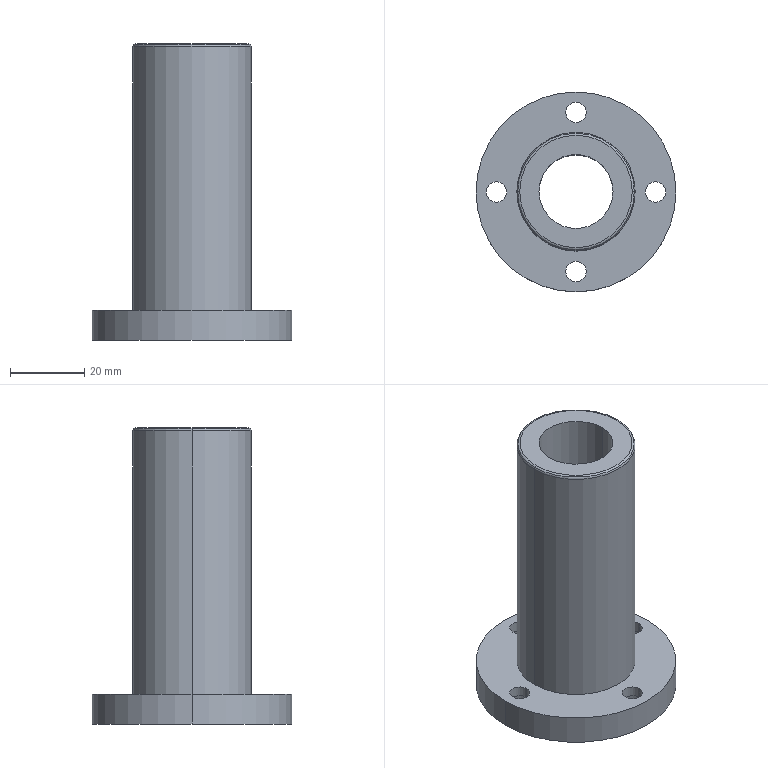Part | NX | features BREP 1 | 1 solid | 33 faces | box 54 x 54 x 80 mm | volume 49508 mm3 | cylinder 22 | plane 7 | torus 4 | commonest cylinder face diameters 5.5 x8 9 x8 20 x2 32 x2 54 x2
STEP:
#1=CARTESIAN_POINT('',(15.2,0.,80.));
#2=VERTEX_POINT('',#1);
#3=CARTESIAN_POINT('',(-15.2,0.,80.));
#4=VERTEX_POINT('',#3);
#5=CARTESIAN_POINT('',(0.,0.,80.));
#6=DIRECTION('',(0.,0.,1.));
#7=DIRECTION('',(1.,0.,0.));
#8=AXIS2_PLACEMENT_3D('',#5,#6,#7);
#9=CIRCLE('',#8,15.2);
#10=EDGE_CURVE('',#2,#4,#9,.T.);
#11=ORIENTED_EDGE('',*,*,#10,.T.);
#12=CARTESIAN_POINT('',(0.,0.,80.));
#13=DIRECTION('',(0.,0.,1.));
#14=DIRECTION('',(-1.,0.,0.));
#15=AXIS2_PLACEMENT_3D('',#12,#13,#14);
#16=CIRCLE('',#15,15.2);
#17=EDGE_CURVE('',#4,#2,#16,.T.);
#18=ORIENTED_EDGE('',*,*,#17,.T.);
#19=EDGE_LOOP('',(#11,#18));
#20=FACE_BOUND('',#19,.T.);
#21=CARTESIAN_POINT('',(10.,0.,80.));
#22=VERTEX_POINT('',#21);
#23=CARTESIAN_POINT('',(-10.,0.,80.));
#24=VERTEX_POINT('',#23);
#25=CARTESIAN_POINT('',(0.,0.,80.));
#26=DIRECTION('',(0.,0.,-1.));
#27=DIRECTION('',(1.,0.,0.));
#28=AXIS2_PLACEMENT_3D('',#25,#26,#27);
#29=CIRCLE('',#28,10.);
#30=EDGE_CURVE('',#22,#24,#29,.T.);
#31=ORIENTED_EDGE('',*,*,#30,.T.);
#32=CARTESIAN_POINT('',(0.,0.,80.));
#33=DIRECTION('',(0.,0.,-1.));
#34=DIRECTION('',(-1.,0.,0.));
#35=AXIS2_PLACEMENT_3D('',#32,#33,#34);
#36=CIRCLE('',#35,10.);
#37=EDGE_CURVE('',#24,#22,#36,.T.);
#38=ORIENTED_EDGE('',*,*,#37,.T.);
#39=EDGE_LOOP('',(#31,#38));
#40=FACE_BOUND('',#39,.T.);
#41=CARTESIAN_POINT('',(0.,15.2,80.));
#42=DIRECTION('',(0.,0.,1.));
#43=DIRECTION('',(1.,0.,0.));
#44=AXIS2_PLACEMENT_3D('',#41,#42,#43);
#45=PLANE('',#44);
#46=ADVANCED_FACE('',(#20,#40),#45,.T.);
#47=CARTESIAN_POINT('',(-15.766,0.,79.766));
#48=VERTEX_POINT('',#47);
#49=CARTESIAN_POINT('',(-15.2,0.,79.2));
#50=DIRECTION('',(0.,-1.,0.));
#51=DIRECTION('',(0.,0.,1.));
#52=AXIS2_PLACEMENT_3D('',#49,#50,#51);
#53=CIRCLE('',#52,0.8);
#54=EDGE_CURVE('',#4,#48,#53,.T.);
#55=ORIENTED_EDGE('',*,*,#54,.T.);
#56=CARTESIAN_POINT('',(15.766,0.,79.766));
#57=VERTEX_POINT('',#56);
#58=CARTESIAN_POINT('',(0.,0.,79.766));
#59=DIRECTION('',(0.,0.,-1.));
#60=DIRECTION('',(1.,0.,0.));
#61=AXIS2_PLACEMENT_3D('',#58,#59,#60);
#62=CIRCLE('',#61,15.766);
#63=EDGE_CURVE('',#57,#48,#62,.T.);
#64=ORIENTED_EDGE('',*,*,#63,.F.);
#65=CARTESIAN_POINT('',(15.2,0.,79.2));
#66=DIRECTION('',(0.,1.,0.));
#67=DIRECTION('',(0.,0.,1.));
#68=AXIS2_PLACEMENT_3D('',#65,#66,#67);
#69=CIRCLE('',#68,0.8);
#70=EDGE_CURVE('',#2,#57,#69,.T.);
#71=ORIENTED_EDGE('',*,*,#70,.F.);
#72=ORIENTED_EDGE('',*,*,#17,.F.);
#73=EDGE_LOOP('',(#55,#64,#71,#72));
#74=FACE_BOUND('',#73,.T.);
#75=CARTESIAN_POINT('',(0.,0.,79.2));
#76=DIRECTION('',(0.,0.,-1.));
#77=DIRECTION('',(-1.,0.,0.));
#78=AXIS2_PLACEMENT_3D('',#75,#76,#77);
#79=TOROIDAL_SURFACE('',#78,15.2,0.8);
#80=ADVANCED_FACE('',(#74),#79,.T.);
#81=ORIENTED_EDGE('',*,*,#70,.T.);
#82=CARTESIAN_POINT('',(0.,0.,79.766));
#83=DIRECTION('',(0.,0.,-1.));
#84=DIRECTION('',(-1.,0.,0.));
#85=AXIS2_PLACEMENT_3D('',#82,#83,#84);
#86=CIRCLE('',#85,15.766);
#87=EDGE_CURVE('',#48,#57,#86,.T.);
#88=ORIENTED_EDGE('',*,*,#87,.F.);
#89=ORIENTED_EDGE('',*,*,#54,.F.);
#90=ORIENTED_EDGE('',*,*,#10,.F.);
#91=EDGE_LOOP('',(#81,#88,#89,#90));
#92=FACE_BOUND('',#91,.T.);
#93=CARTESIAN_POINT('',(0.,0.,79.2));
#94=DIRECTION('',(0.,0.,-1.));
#95=DIRECTION('',(-1.,0.,0.));
#96=AXIS2_PLACEMENT_3D('',#93,#94,#95);
#97=TOROIDAL_SURFACE('',#96,15.2,0.8);
#98=ADVANCED_FACE('',(#92),#97,.T.);
#99=CARTESIAN_POINT('',(-16.,0.,79.2));
#100=VERTEX_POINT('',#99);
#101=CARTESIAN_POINT('',(-15.2,0.,79.2));
#102=DIRECTION('',(0.,-1.,0.));
#103=DIRECTION('',(-0.7071,0.,0.7071));
#104=AXIS2_PLACEMENT_3D('',#101,#102,#103);
#105=CIRCLE('',#104,0.8);
#106=EDGE_CURVE('',#48,#100,#105,.T.);
#107=ORIENTED_EDGE('',*,*,#106,.F.);
#108=ORIENTED_EDGE('',*,*,#87,.T.);
#109=CARTESIAN_POINT('',(16.,0.,79.2));
#110=VERTEX_POINT('',#109);
#111=CARTESIAN_POINT('',(15.2,0.,79.2));
#112=DIRECTION('',(0.,1.,0.));
#113=DIRECTION('',(0.7071,0.,0.7071));
#114=AXIS2_PLACEMENT_3D('',#111,#112,#113);
#115=CIRCLE('',#114,0.8);
#116=EDGE_CURVE('',#57,#110,#115,.T.);
#117=ORIENTED_EDGE('',*,*,#116,.T.);
#118=CARTESIAN_POINT('',(0.,0.,79.2));
#119=DIRECTION('',(0.,0.,1.));
#120=DIRECTION('',(1.,0.,0.));
#121=AXIS2_PLACEMENT_3D('',#118,#119,#120);
#122=CIRCLE('',#121,16.);
#123=EDGE_CURVE('',#110,#100,#122,.T.);
#124=ORIENTED_EDGE('',*,*,#123,.T.);
#125=EDGE_LOOP('',(#107,#108,#117,#124));
#126=FACE_BOUND('',#125,.T.);
#127=CARTESIAN_POINT('',(0.,0.,79.2));
#128=DIRECTION('',(0.,0.,-1.));
#129=DIRECTION('',(-1.,0.,0.));
#130=AXIS2_PLACEMENT_3D('',#127,#128,#129);
#131=TOROIDAL_SURFACE('',#130,15.2,0.8);
#132=ADVANCED_FACE('',(#126),#131,.T.);
#133=CARTESIAN_POINT('',(-16.,0.,8.));
#134=VERTEX_POINT('',#133);
#135=CARTESIAN_POINT('',(-16.,0.,8.));
#136=DIRECTION('',(0.,0.,1.));
#137=VECTOR('',#136,1000.);
#138=LINE('',#135,#137);
#139=EDGE_CURVE('',#134,#100,#138,.T.);
#140=ORIENTED_EDGE('',*,*,#139,.T.);
#141=ORIENTED_EDGE('',*,*,#123,.F.);
#142=CARTESIAN_POINT('',(16.,0.,8.));
#143=VERTEX_POINT('',#142);
#144=CARTESIAN_POINT('',(16.,0.,8.));
#145=DIRECTION('',(0.,0.,1.));
#146=VECTOR('',#145,1000.);
#147=LINE('',#144,#146);
#148=EDGE_CURVE('',#143,#110,#147,.T.);
#149=ORIENTED_EDGE('',*,*,#148,.F.);
#150=CARTESIAN_POINT('',(0.,0.,8.));
#151=DIRECTION('',(0.,0.,-1.));
#152=DIRECTION('',(-1.,0.,0.));
#153=AXIS2_PLACEMENT_3D('',#150,#151,#152);
#154=CIRCLE('',#153,16.);
#155=EDGE_CURVE('',#134,#143,#154,.T.);
#156=ORIENTED_EDGE('',*,*,#155,.F.);
#157=EDGE_LOOP('',(#140,#141,#149,#156));
#158=FACE_BOUND('',#157,.T.);
#159=CARTESIAN_POINT('',(0.,0.,0.));
#160=DIRECTION('',(0.,0.,1.));
#161=DIRECTION('',(-1.,0.,0.));
#162=AXIS2_PLACEMENT_3D('',#159,#160,#161);
#163=CYLINDRICAL_SURFACE('',#162,16.);
#164=ADVANCED_FACE('',(#158),#163,.T.);
#165=CARTESIAN_POINT('',(-27.,0.,8.));
#166=VERTEX_POINT('',#165);
#167=CARTESIAN_POINT('',(27.,0.,8.));
#168=VERTEX_POINT('',#167);
#169=CARTESIAN_POINT('',(0.,0.,8.));
#170=DIRECTION('',(0.,0.,1.));
#171=DIRECTION('',(-1.,0.,0.));
#172=AXIS2_PLACEMENT_3D('',#169,#170,#171);
#173=CIRCLE('',#172,27.);
#174=EDGE_CURVE('',#166,#168,#173,.T.);
#175=ORIENTED_EDGE('',*,*,#174,.T.);
#176=CARTESIAN_POINT('',(0.,0.,8.));
#177=DIRECTION('',(0.,0.,1.));
#178=DIRECTION('',(1.,0.,0.));
#179=AXIS2_PLACEMENT_3D('',#176,#177,#178);
#180=CIRCLE('',#179,27.);
#181=EDGE_CURVE('',#168,#166,#180,.T.);
#182=ORIENTED_EDGE('',*,*,#181,.T.);
#183=EDGE_LOOP('',(#175,#182));
#184=FACE_BOUND('',#183,.T.);
#185=CARTESIAN_POINT('',(18.75,0.,8.));
#186=VERTEX_POINT('',#185);
#187=CARTESIAN_POINT('',(24.25,0.,8.));
#188=VERTEX_POINT('',#187);
#189=CARTESIAN_POINT('',(21.5,0.,8.));
#190=DIRECTION('',(0.,0.,-1.));
#191=DIRECTION('',(-1.,0.,0.));
#192=AXIS2_PLACEMENT_3D('',#189,#190,#191);
#193=CIRCLE('',#192,2.75);
#194=EDGE_CURVE('',#186,#188,#193,.T.);
#195=ORIENTED_EDGE('',*,*,#194,.T.);
#196=CARTESIAN_POINT('',(21.5,0.,8.));
#197=DIRECTION('',(0.,0.,-1.));
#198=DIRECTION('',(1.,0.,0.));
#199=AXIS2_PLACEMENT_3D('',#196,#197,#198);
#200=CIRCLE('',#199,2.75);
#201=EDGE_CURVE('',#188,#186,#200,.T.);
#202=ORIENTED_EDGE('',*,*,#201,.T.);
#203=EDGE_LOOP('',(#195,#202));
#204=FACE_BOUND('',#203,.T.);
#205=CARTESIAN_POINT('',(-18.75,0.,8.));
#206=VERTEX_POINT('',#205);
#207=CARTESIAN_POINT('',(-24.25,0.,8.));
#208=VERTEX_POINT('',#207);
#209=CARTESIAN_POINT('',(-21.5,0.,8.));
#210=DIRECTION('',(0.,0.,-1.));
#211=DIRECTION('',(1.,0.,0.));
#212=AXIS2_PLACEMENT_3D('',#209,#210,#211);
#213=CIRCLE('',#212,2.75);
#214=EDGE_CURVE('',#206,#208,#213,.T.);
#215=ORIENTED_EDGE('',*,*,#214,.T.);
#216=CARTESIAN_POINT('',(-21.5,0.,8.));
#217=DIRECTION('',(0.,0.,-1.));
#218=DIRECTION('',(-1.,0.,0.));
#219=AXIS2_PLACEMENT_3D('',#216,#217,#218);
#220=CIRCLE('',#219,2.75);
#221=EDGE_CURVE('',#208,#206,#220,.T.);
#222=ORIENTED_EDGE('',*,*,#221,.T.);
#223=EDGE_LOOP('',(#215,#222));
#224=FACE_BOUND('',#223,.T.);
#225=CARTESIAN_POINT('',(-2.75,-21.5,8.));
#226=VERTEX_POINT('',#225);
#227=CARTESIAN_POINT('',(2.75,-21.5,8.));
#228=VERTEX_POINT('',#227);
#229=CARTESIAN_POINT('',(0.,-21.5,8.));
#230=DIRECTION('',(0.,0.,-1.));
#231=DIRECTION('',(-1.,0.,0.));
#232=AXIS2_PLACEMENT_3D('',#229,#230,#231);
#233=CIRCLE('',#232,2.75);
#234=EDGE_CURVE('',#226,#228,#233,.T.);
#235=ORIENTED_EDGE('',*,*,#234,.T.);
#236=CARTESIAN_POINT('',(0.,-21.5,8.));
#237=DIRECTION('',(0.,0.,-1.));
#238=DIRECTION('',(1.,0.,0.));
#239=AXIS2_PLACEMENT_3D('',#236,#237,#238);
#240=CIRCLE('',#239,2.75);
#241=EDGE_CURVE('',#228,#226,#240,.T.);
#242=ORIENTED_EDGE('',*,*,#241,.T.);
#243=EDGE_LOOP('',(#235,#242));
#244=FACE_BOUND('',#243,.T.);
#245=CARTESIAN_POINT('',(2.75,21.5,8.));
#246=VERTEX_POINT('',#245);
#247=CARTESIAN_POINT('',(-2.75,21.5,8.));
#248=VERTEX_POINT('',#247);
#249=CARTESIAN_POINT('',(0.,21.5,8.));
#250=DIRECTION('',(0.,0.,-1.));
#251=DIRECTION('',(1.,0.,0.));
#252=AXIS2_PLACEMENT_3D('',#249,#250,#251);
#253=CIRCLE('',#252,2.75);
#254=EDGE_CURVE('',#246,#248,#253,.T.);
#255=ORIENTED_EDGE('',*,*,#254,.T.);
#256=CARTESIAN_POINT('',(0.,21.5,8.));
#257=DIRECTION('',(0.,0.,-1.));
#258=DIRECTION('',(-1.,0.,0.));
#259=AXIS2_PLACEMENT_3D('',#256,#257,#258);
#260=CIRCLE('',#259,2.75);
#261=EDGE_CURVE('',#248,#246,#260,.T.);
#262=ORIENTED_EDGE('',*,*,#261,.T.);
#263=EDGE_LOOP('',(#255,#262));
#264=FACE_BOUND('',#263,.T.);
#265=ORIENTED_EDGE('',*,*,#155,.T.);
#266=CARTESIAN_POINT('',(0.,0.,8.));
#267=DIRECTION('',(0.,0.,-1.));
#268=DIRECTION('',(1.,0.,0.));
#269=AXIS2_PLACEMENT_3D('',#266,#267,#268);
#270=CIRCLE('',#269,16.);
#271=EDGE_CURVE('',#143,#134,#270,.T.);
#272=ORIENTED_EDGE('',*,*,#271,.T.);
#273=EDGE_LOOP('',(#265,#272));
#274=FACE_BOUND('',#273,.T.);
#275=CARTESIAN_POINT('',(0.,0.,8.));
#276=DIRECTION('',(0.,0.,1.));
#277=DIRECTION('',(1.,0.,0.));
#278=AXIS2_PLACEMENT_3D('',#275,#276,#277);
#279=PLANE('',#278);
#280=ADVANCED_FACE('',(#184,#204,#224,#244,#264,#274),#279,.T.);
#281=CARTESIAN_POINT('',(-27.,0.,0.));
#282=VERTEX_POINT('',#281);
#283=CARTESIAN_POINT('',(-27.,0.,0.));
#284=DIRECTION('',(0.,0.,1.));
#285=VECTOR('',#284,1000.);
#286=LINE('',#283,#285);
#287=EDGE_CURVE('',#282,#166,#286,.T.);
#288=ORIENTED_EDGE('',*,*,#287,.T.);
#289=ORIENTED_EDGE('',*,*,#181,.F.);
#290=CARTESIAN_POINT('',(27.,0.,0.));
#291=VERTEX_POINT('',#290);
#292=CARTESIAN_POINT('',(27.,0.,0.));
#293=DIRECTION('',(0.,0.,1.));
#294=VECTOR('',#293,1000.);
#295=LINE('',#292,#294);
#296=EDGE_CURVE('',#291,#168,#295,.T.);
#297=ORIENTED_EDGE('',*,*,#296,.F.);
#298=CARTESIAN_POINT('',(0.,0.,0.));
#299=DIRECTION('',(0.,0.,-1.));
#300=DIRECTION('',(-1.,0.,0.));
#301=AXIS2_PLACEMENT_3D('',#298,#299,#300);
#302=CIRCLE('',#301,27.);
#303=EDGE_CURVE('',#282,#291,#302,.T.);
#304=ORIENTED_EDGE('',*,*,#303,.F.);
#305=EDGE_LOOP('',(#288,#289,#297,#304));
#306=FACE_BOUND('',#305,.T.);
#307=CARTESIAN_POINT('',(0.,0.,8.));
#308=DIRECTION('',(0.,0.,1.));
#309=DIRECTION('',(-1.,0.,0.));
#310=AXIS2_PLACEMENT_3D('',#307,#308,#309);
#311=CYLINDRICAL_SURFACE('',#310,27.);
#312=ADVANCED_FACE('',(#306),#311,.T.);
#313=ORIENTED_EDGE('',*,*,#303,.T.);
#314=CARTESIAN_POINT('',(0.,0.,0.));
#315=DIRECTION('',(0.,0.,-1.));
#316=DIRECTION('',(1.,0.,0.));
#317=AXIS2_PLACEMENT_3D('',#314,#315,#316);
#318=CIRCLE('',#317,27.);
#319=EDGE_CURVE('',#291,#282,#318,.T.);
#320=ORIENTED_EDGE('',*,*,#319,.T.);
#321=EDGE_LOOP('',(#313,#320));
#322=FACE_BOUND('',#321,.T.);
#323=CARTESIAN_POINT('',(17.,0.,0.));
#324=VERTEX_POINT('',#323);
#325=CARTESIAN_POINT('',(26.,0.,0.));
#326=VERTEX_POINT('',#325);
#327=CARTESIAN_POINT('',(21.5,0.,0.));
#328=DIRECTION('',(0.,0.,1.));
#329=DIRECTION('',(-1.,0.,0.));
#330=AXIS2_PLACEMENT_3D('',#327,#328,#329);
#331=CIRCLE('',#330,4.5);
#332=EDGE_CURVE('',#324,#326,#331,.T.);
#333=ORIENTED_EDGE('',*,*,#332,.T.);
#334=CARTESIAN_POINT('',(21.5,0.,0.));
#335=DIRECTION('',(0.,0.,1.));
#336=DIRECTION('',(1.,0.,0.));
#337=AXIS2_PLACEMENT_3D('',#334,#335,#336);
#338=CIRCLE('',#337,4.5);
#339=EDGE_CURVE('',#326,#324,#338,.T.);
#340=ORIENTED_EDGE('',*,*,#339,.T.);
#341=EDGE_LOOP('',(#333,#340));
#342=FACE_BOUND('',#341,.T.);
#343=CARTESIAN_POINT('',(-17.,0.,0.));
#344=VERTEX_POINT('',#343);
#345=CARTESIAN_POINT('',(-26.,0.,0.));
#346=VERTEX_POINT('',#345);
#347=CARTESIAN_POINT('',(-21.5,0.,0.));
#348=DIRECTION('',(0.,0.,1.));
#349=DIRECTION('',(1.,0.,0.));
#350=AXIS2_PLACEMENT_3D('',#347,#348,#349);
#351=CIRCLE('',#350,4.5);
#352=EDGE_CURVE('',#344,#346,#351,.T.);
#353=ORIENTED_EDGE('',*,*,#352,.T.);
#354=CARTESIAN_POINT('',(-21.5,0.,0.));
#355=DIRECTION('',(0.,0.,1.));
#356=DIRECTION('',(-1.,0.,0.));
#357=AXIS2_PLACEMENT_3D('',#354,#355,#356);
#358=CIRCLE('',#357,4.5);
#359=EDGE_CURVE('',#346,#344,#358,.T.);
#360=ORIENTED_EDGE('',*,*,#359,.T.);
#361=EDGE_LOOP('',(#353,#360));
#362=FACE_BOUND('',#361,.T.);
#363=CARTESIAN_POINT('',(-4.5,-21.5,0.));
#364=VERTEX_POINT('',#363);
#365=CARTESIAN_POINT('',(4.5,-21.5,0.));
#366=VERTEX_POINT('',#365);
#367=CARTESIAN_POINT('',(0.,-21.5,0.));
#368=DIRECTION('',(0.,0.,1.));
#369=DIRECTION('',(-1.,0.,0.));
#370=AXIS2_PLACEMENT_3D('',#367,#368,#369);
#371=CIRCLE('',#370,4.5);
#372=EDGE_CURVE('',#364,#366,#371,.T.);
#373=ORIENTED_EDGE('',*,*,#372,.T.);
#374=CARTESIAN_POINT('',(0.,-21.5,0.));
#375=DIRECTION('',(0.,0.,1.));
#376=DIRECTION('',(1.,0.,0.));
#377=AXIS2_PLACEMENT_3D('',#374,#375,#376);
#378=CIRCLE('',#377,4.5);
#379=EDGE_CURVE('',#366,#364,#378,.T.);
#380=ORIENTED_EDGE('',*,*,#379,.T.);
#381=EDGE_LOOP('',(#373,#380));
#382=FACE_BOUND('',#381,.T.);
#383=CARTESIAN_POINT('',(4.5,21.5,0.));
#384=VERTEX_POINT('',#383);
#385=CARTESIAN_POINT('',(-4.5,21.5,0.));
#386=VERTEX_POINT('',#385);
#387=CARTESIAN_POINT('',(0.,21.5,0.));
#388=DIRECTION('',(0.,0.,1.));
#389=DIRECTION('',(1.,0.,0.));
#390=AXIS2_PLACEMENT_3D('',#387,#388,#389);
#391=CIRCLE('',#390,4.5);
#392=EDGE_CURVE('',#384,#386,#391,.T.);
#393=ORIENTED_EDGE('',*,*,#392,.T.);
#394=CARTESIAN_POINT('',(0.,21.5,0.));
#395=DIRECTION('',(0.,0.,1.));
#396=DIRECTION('',(-1.,0.,0.));
#397=AXIS2_PLACEMENT_3D('',#394,#395,#396);
#398=CIRCLE('',#397,4.5);
#399=EDGE_CURVE('',#386,#384,#398,.T.);
#400=ORIENTED_EDGE('',*,*,#399,.T.);
#401=EDGE_LOOP('',(#393,#400));
#402=FACE_BOUND('',#401,.T.);
#403=CARTESIAN_POINT('',(10.,0.,0.));
#404=VERTEX_POINT('',#403);
#405=CARTESIAN_POINT('',(-10.,0.,0.));
#406=VERTEX_POINT('',#405);
#407=CARTESIAN_POINT('',(0.,0.,0.));
#408=DIRECTION('',(0.,0.,1.));
#409=DIRECTION('',(1.,0.,0.));
#410=AXIS2_PLACEMENT_3D('',#407,#408,#409);
#411=CIRCLE('',#410,10.);
#412=EDGE_CURVE('',#404,#406,#411,.T.);
#413=ORIENTED_EDGE('',*,*,#412,.T.);
#414=CARTESIAN_POINT('',(0.,0.,0.));
#415=DIRECTION('',(0.,0.,1.));
#416=DIRECTION('',(-1.,0.,0.));
#417=AXIS2_PLACEMENT_3D('',#414,#415,#416);
#418=CIRCLE('',#417,10.);
#419=EDGE_CURVE('',#406,#404,#418,.T.);
#420=ORIENTED_EDGE('',*,*,#419,.T.);
#421=EDGE_LOOP('',(#413,#420));
#422=FACE_BOUND('',#421,.T.);
#423=CARTESIAN_POINT('',(0.,10.,0.));
#424=DIRECTION('',(0.,0.,-1.));
#425=DIRECTION('',(0.,-1.,0.));
#426=AXIS2_PLACEMENT_3D('',#423,#424,#425);
#427=PLANE('',#426);
#428=ADVANCED_FACE('',(#322,#342,#362,#382,#402,#422),#427,.T.);
#429=ORIENTED_EDGE('',*,*,#296,.T.);
#430=ORIENTED_EDGE('',*,*,#174,.F.);
#431=ORIENTED_EDGE('',*,*,#287,.F.);
#432=ORIENTED_EDGE('',*,*,#319,.F.);
#433=EDGE_LOOP('',(#429,#430,#431,#432));
#434=FACE_BOUND('',#433,.T.);
#435=CARTESIAN_POINT('',(0.,0.,8.));
#436=DIRECTION('',(0.,0.,1.));
#437=DIRECTION('',(-1.,0.,0.));
#438=AXIS2_PLACEMENT_3D('',#435,#436,#437);
#439=CYLINDRICAL_SURFACE('',#438,27.);
#440=ADVANCED_FACE('',(#434),#439,.T.);
#441=CARTESIAN_POINT('',(26.,0.,5.1));
#442=VERTEX_POINT('',#441);
#443=CARTESIAN_POINT('',(26.,0.,5.1));
#444=DIRECTION('',(0.,0.,-1.));
#445=VECTOR('',#444,1000.);
#446=LINE('',#443,#445);
#447=EDGE_CURVE('',#326,#442,#446,.F.);
#448=ORIENTED_EDGE('',*,*,#447,.T.);
#449=CARTESIAN_POINT('',(17.,0.,5.1));
#450=VERTEX_POINT('',#449);
#451=CARTESIAN_POINT('',(21.5,0.,5.1));
#452=DIRECTION('',(0.,0.,-1.));
#453=DIRECTION('',(-1.,0.,0.));
#454=AXIS2_PLACEMENT_3D('',#451,#452,#453);
#455=CIRCLE('',#454,4.5);
#456=EDGE_CURVE('',#450,#442,#455,.T.);
#457=ORIENTED_EDGE('',*,*,#456,.F.);
#458=CARTESIAN_POINT('',(17.,0.,5.1));
#459=DIRECTION('',(0.,0.,-1.));
#460=VECTOR('',#459,1000.);
#461=LINE('',#458,#460);
#462=EDGE_CURVE('',#324,#450,#461,.F.);
#463=ORIENTED_EDGE('',*,*,#462,.F.);
#464=ORIENTED_EDGE('',*,*,#339,.F.);
#465=EDGE_LOOP('',(#448,#457,#463,#464));
#466=FACE_BOUND('',#465,.T.);
#467=CARTESIAN_POINT('',(21.5,0.,8.));
#468=DIRECTION('',(0.,0.,-1.));
#469=DIRECTION('',(1.,0.,0.));
#470=AXIS2_PLACEMENT_3D('',#467,#468,#469);
#471=CYLINDRICAL_SURFACE('',#470,4.5);
#472=ADVANCED_FACE('',(#466),#471,.F.);
#473=ORIENTED_EDGE('',*,*,#462,.T.);
#474=CARTESIAN_POINT('',(21.5,0.,5.1));
#475=DIRECTION('',(0.,0.,-1.));
#476=DIRECTION('',(1.,0.,0.));
#477=AXIS2_PLACEMENT_3D('',#474,#475,#476);
#478=CIRCLE('',#477,4.5);
#479=EDGE_CURVE('',#442,#450,#478,.T.);
#480=ORIENTED_EDGE('',*,*,#479,.F.);
#481=ORIENTED_EDGE('',*,*,#447,.F.);
#482=ORIENTED_EDGE('',*,*,#332,.F.);
#483=EDGE_LOOP('',(#473,#480,#481,#482));
#484=FACE_BOUND('',#483,.T.);
#485=CARTESIAN_POINT('',(21.5,0.,8.));
#486=DIRECTION('',(0.,0.,-1.));
#487=DIRECTION('',(1.,0.,0.));
#488=AXIS2_PLACEMENT_3D('',#485,#486,#487);
#489=CYLINDRICAL_SURFACE('',#488,4.5);
#490=ADVANCED_FACE('',(#484),#489,.F.);
#491=ORIENTED_EDGE('',*,*,#456,.T.);
#492=ORIENTED_EDGE('',*,*,#479,.T.);
#493=EDGE_LOOP('',(#491,#492));
#494=FACE_BOUND('',#493,.T.);
#495=CARTESIAN_POINT('',(18.75,0.,5.1));
#496=VERTEX_POINT('',#495);
#497=CARTESIAN_POINT('',(24.25,0.,5.1));
#498=VERTEX_POINT('',#497);
#499=CARTESIAN_POINT('',(21.5,0.,5.1));
#500=DIRECTION('',(0.,0.,1.));
#501=DIRECTION('',(-1.,0.,0.));
#502=AXIS2_PLACEMENT_3D('',#499,#500,#501);
#503=CIRCLE('',#502,2.75);
#504=EDGE_CURVE('',#496,#498,#503,.T.);
#505=ORIENTED_EDGE('',*,*,#504,.T.);
#506=CARTESIAN_POINT('',(21.5,0.,5.1));
#507=DIRECTION('',(0.,0.,1.));
#508=DIRECTION('',(1.,0.,0.));
#509=AXIS2_PLACEMENT_3D('',#506,#507,#508);
#510=CIRCLE('',#509,2.75);
#511=EDGE_CURVE('',#498,#496,#510,.T.);
#512=ORIENTED_EDGE('',*,*,#511,.T.);
#513=EDGE_LOOP('',(#505,#512));
#514=FACE_BOUND('',#513,.T.);
#515=CARTESIAN_POINT('',(26.,0.,5.1));
#516=DIRECTION('',(0.,0.,-1.));
#517=DIRECTION('',(0.,-1.,0.));
#518=AXIS2_PLACEMENT_3D('',#515,#516,#517);
#519=PLANE('',#518);
#520=ADVANCED_FACE('',(#494,#514),#519,.T.);
#521=CARTESIAN_POINT('',(24.25,0.,8.));
#522=DIRECTION('',(0.,0.,-1.));
#523=VECTOR('',#522,1000.);
#524=LINE('',#521,#523);
#525=EDGE_CURVE('',#498,#188,#524,.F.);
#526=ORIENTED_EDGE('',*,*,#525,.T.);
#527=ORIENTED_EDGE('',*,*,#194,.F.);
#528=CARTESIAN_POINT('',(18.75,0.,8.));
#529=DIRECTION('',(0.,0.,-1.));
#530=VECTOR('',#529,1000.);
#531=LINE('',#528,#530);
#532=EDGE_CURVE('',#496,#186,#531,.F.);
#533=ORIENTED_EDGE('',*,*,#532,.F.);
#534=ORIENTED_EDGE('',*,*,#511,.F.);
#535=EDGE_LOOP('',(#526,#527,#533,#534));
#536=FACE_BOUND('',#535,.T.);
#537=CARTESIAN_POINT('',(21.5,0.,8.));
#538=DIRECTION('',(0.,0.,-1.));
#539=DIRECTION('',(1.,0.,0.));
#540=AXIS2_PLACEMENT_3D('',#537,#538,#539);
#541=CYLINDRICAL_SURFACE('',#540,2.75);
#542=ADVANCED_FACE('',(#536),#541,.F.);
#543=ORIENTED_EDGE('',*,*,#532,.T.);
#544=ORIENTED_EDGE('',*,*,#201,.F.);
#545=ORIENTED_EDGE('',*,*,#525,.F.);
#546=ORIENTED_EDGE('',*,*,#504,.F.);
#547=EDGE_LOOP('',(#543,#544,#545,#546));
#548=FACE_BOUND('',#547,.T.);
#549=CARTESIAN_POINT('',(21.5,0.,8.));
#550=DIRECTION('',(0.,0.,-1.));
#551=DIRECTION('',(1.,0.,0.));
#552=AXIS2_PLACEMENT_3D('',#549,#550,#551);
#553=CYLINDRICAL_SURFACE('',#552,2.75);
#554=ADVANCED_FACE('',(#548),#553,.F.);
#555=CARTESIAN_POINT('',(-17.,0.,5.1));
#556=VERTEX_POINT('',#555);
#557=CARTESIAN_POINT('',(-17.,0.,0.));
#558=DIRECTION('',(0.,0.,1.));
#559=VECTOR('',#558,1000.);
#560=LINE('',#557,#559);
#561=EDGE_CURVE('',#556,#344,#560,.F.);
#562=ORIENTED_EDGE('',*,*,#561,.T.);
#563=ORIENTED_EDGE('',*,*,#359,.F.);
#564=CARTESIAN_POINT('',(-26.,0.,5.1));
#565=VERTEX_POINT('',#564);
#566=CARTESIAN_POINT('',(-26.,0.,0.));
#567=DIRECTION('',(0.,0.,1.));
#568=VECTOR('',#567,1000.);
#569=LINE('',#566,#568);
#570=EDGE_CURVE('',#565,#346,#569,.F.);
#571=ORIENTED_EDGE('',*,*,#570,.F.);
#572=CARTESIAN_POINT('',(-21.5,0.,5.1));
#573=DIRECTION('',(0.,0.,-1.));
#574=DIRECTION('',(1.,0.,0.));
#575=AXIS2_PLACEMENT_3D('',#572,#573,#574);
#576=CIRCLE('',#575,4.5);
#577=EDGE_CURVE('',#556,#565,#576,.T.);
#578=ORIENTED_EDGE('',*,*,#577,.F.);
#579=EDGE_LOOP('',(#562,#563,#571,#578));
#580=FACE_BOUND('',#579,.T.);
#581=CARTESIAN_POINT('',(-21.5,0.,0.));
#582=DIRECTION('',(0.,0.,1.));
#583=DIRECTION('',(-1.,0.,0.));
#584=AXIS2_PLACEMENT_3D('',#581,#582,#583);
#585=CYLINDRICAL_SURFACE('',#584,4.5);
#586=ADVANCED_FACE('',(#580),#585,.F.);
#587=ORIENTED_EDGE('',*,*,#577,.T.);
#588=CARTESIAN_POINT('',(-21.5,0.,5.1));
#589=DIRECTION('',(0.,0.,-1.));
#590=DIRECTION('',(-1.,0.,0.));
#591=AXIS2_PLACEMENT_3D('',#588,#589,#590);
#592=CIRCLE('',#591,4.5);
#593=EDGE_CURVE('',#565,#556,#592,.T.);
#594=ORIENTED_EDGE('',*,*,#593,.T.);
#595=EDGE_LOOP('',(#587,#594));
#596=FACE_BOUND('',#595,.T.);
#597=CARTESIAN_POINT('',(-18.75,0.,5.1));
#598=VERTEX_POINT('',#597);
#599=CARTESIAN_POINT('',(-24.25,0.,5.1));
#600=VERTEX_POINT('',#599);
#601=CARTESIAN_POINT('',(-21.5,0.,5.1));
#602=DIRECTION('',(0.,0.,1.));
#603=DIRECTION('',(1.,0.,0.));
#604=AXIS2_PLACEMENT_3D('',#601,#602,#603);
#605=CIRCLE('',#604,2.75);
#606=EDGE_CURVE('',#598,#600,#605,.T.);
#607=ORIENTED_EDGE('',*,*,#606,.T.);
#608=CARTESIAN_POINT('',(-21.5,0.,5.1));
#609=DIRECTION('',(0.,0.,1.));
#610=DIRECTION('',(-1.,0.,0.));
#611=AXIS2_PLACEMENT_3D('',#608,#609,#610);
#612=CIRCLE('',#611,2.75);
#613=EDGE_CURVE('',#600,#598,#612,.T.);
#614=ORIENTED_EDGE('',*,*,#613,.T.);
#615=EDGE_LOOP('',(#607,#614));
#616=FACE_BOUND('',#615,.T.);
#617=CARTESIAN_POINT('',(-24.25,0.,5.1));
#618=DIRECTION('',(0.,0.,-1.));
#619=DIRECTION('',(0.,-1.,0.));
#620=AXIS2_PLACEMENT_3D('',#617,#618,#619);
#621=PLANE('',#620);
#622=ADVANCED_FACE('',(#596,#616),#621,.T.);
#623=ORIENTED_EDGE('',*,*,#570,.T.);
#624=ORIENTED_EDGE('',*,*,#352,.F.);
#625=ORIENTED_EDGE('',*,*,#561,.F.);
#626=ORIENTED_EDGE('',*,*,#593,.F.);
#627=EDGE_LOOP('',(#623,#624,#625,#626));
#628=FACE_BOUND('',#627,.T.);
#629=CARTESIAN_POINT('',(-21.5,0.,0.));
#630=DIRECTION('',(0.,0.,1.));
#631=DIRECTION('',(-1.,0.,0.));
#632=AXIS2_PLACEMENT_3D('',#629,#630,#631);
#633=CYLINDRICAL_SURFACE('',#632,4.5);
#634=ADVANCED_FACE('',(#628),#633,.F.);
#635=CARTESIAN_POINT('',(-18.75,0.,5.1));
#636=DIRECTION('',(0.,0.,1.));
#637=VECTOR('',#636,1000.);
#638=LINE('',#635,#637);
#639=EDGE_CURVE('',#206,#598,#638,.F.);
#640=ORIENTED_EDGE('',*,*,#639,.T.);
#641=ORIENTED_EDGE('',*,*,#613,.F.);
#642=CARTESIAN_POINT('',(-24.25,0.,5.1));
#643=DIRECTION('',(0.,0.,1.));
#644=VECTOR('',#643,1000.);
#645=LINE('',#642,#644);
#646=EDGE_CURVE('',#208,#600,#645,.F.);
#647=ORIENTED_EDGE('',*,*,#646,.F.);
#648=ORIENTED_EDGE('',*,*,#214,.F.);
#649=EDGE_LOOP('',(#640,#641,#647,#648));
#650=FACE_BOUND('',#649,.T.);
#651=CARTESIAN_POINT('',(-21.5,0.,0.));
#652=DIRECTION('',(0.,0.,1.));
#653=DIRECTION('',(-1.,0.,0.));
#654=AXIS2_PLACEMENT_3D('',#651,#652,#653);
#655=CYLINDRICAL_SURFACE('',#654,2.75);
#656=ADVANCED_FACE('',(#650),#655,.F.);
#657=ORIENTED_EDGE('',*,*,#646,.T.);
#658=ORIENTED_EDGE('',*,*,#606,.F.);
#659=ORIENTED_EDGE('',*,*,#639,.F.);
#660=ORIENTED_EDGE('',*,*,#221,.F.);
#661=EDGE_LOOP('',(#657,#658,#659,#660));
#662=FACE_BOUND('',#661,.T.);
#663=CARTESIAN_POINT('',(-21.5,0.,0.));
#664=DIRECTION('',(0.,0.,1.));
#665=DIRECTION('',(-1.,0.,0.));
#666=AXIS2_PLACEMENT_3D('',#663,#664,#665);
#667=CYLINDRICAL_SURFACE('',#666,2.75);
#668=ADVANCED_FACE('',(#662),#667,.F.);
#669=CARTESIAN_POINT('',(4.5,-21.5,5.1));
#670=VERTEX_POINT('',#669);
#671=CARTESIAN_POINT('',(4.5,-21.5,5.1));
#672=DIRECTION('',(0.,0.,-1.));
#673=VECTOR('',#672,1000.);
#674=LINE('',#671,#673);
#675=EDGE_CURVE('',#366,#670,#674,.F.);
#676=ORIENTED_EDGE('',*,*,#675,.T.);
#677=CARTESIAN_POINT('',(-4.5,-21.5,5.1));
#678=VERTEX_POINT('',#677);
#679=CARTESIAN_POINT('',(0.,-21.5,5.1));
#680=DIRECTION('',(0.,0.,-1.));
#681=DIRECTION('',(-1.,0.,0.));
#682=AXIS2_PLACEMENT_3D('',#679,#680,#681);
#683=CIRCLE('',#682,4.5);
#684=EDGE_CURVE('',#678,#670,#683,.T.);
#685=ORIENTED_EDGE('',*,*,#684,.F.);
#686=CARTESIAN_POINT('',(-4.5,-21.5,5.1));
#687=DIRECTION('',(0.,0.,-1.));
#688=VECTOR('',#687,1000.);
#689=LINE('',#686,#688);
#690=EDGE_CURVE('',#364,#678,#689,.F.);
#691=ORIENTED_EDGE('',*,*,#690,.F.);
#692=ORIENTED_EDGE('',*,*,#379,.F.);
#693=EDGE_LOOP('',(#676,#685,#691,#692));
#694=FACE_BOUND('',#693,.T.);
#695=CARTESIAN_POINT('',(0.,-21.5,8.));
#696=DIRECTION('',(0.,0.,-1.));
#697=DIRECTION('',(1.,0.,0.));
#698=AXIS2_PLACEMENT_3D('',#695,#696,#697);
#699=CYLINDRICAL_SURFACE('',#698,4.5);
#700=ADVANCED_FACE('',(#694),#699,.F.);
#701=ORIENTED_EDGE('',*,*,#690,.T.);
#702=CARTESIAN_POINT('',(0.,-21.5,5.1));
#703=DIRECTION('',(0.,0.,-1.));
#704=DIRECTION('',(1.,0.,0.));
#705=AXIS2_PLACEMENT_3D('',#702,#703,#704);
#706=CIRCLE('',#705,4.5);
#707=EDGE_CURVE('',#670,#678,#706,.T.);
#708=ORIENTED_EDGE('',*,*,#707,.F.);
#709=ORIENTED_EDGE('',*,*,#675,.F.);
#710=ORIENTED_EDGE('',*,*,#372,.F.);
#711=EDGE_LOOP('',(#701,#708,#709,#710));
#712=FACE_BOUND('',#711,.T.);
#713=CARTESIAN_POINT('',(0.,-21.5,8.));
#714=DIRECTION('',(0.,0.,-1.));
#715=DIRECTION('',(1.,0.,0.));
#716=AXIS2_PLACEMENT_3D('',#713,#714,#715);
#717=CYLINDRICAL_SURFACE('',#716,4.5);
#718=ADVANCED_FACE('',(#712),#717,.F.);
#719=ORIENTED_EDGE('',*,*,#684,.T.);
#720=ORIENTED_EDGE('',*,*,#707,.T.);
#721=EDGE_LOOP('',(#719,#720));
#722=FACE_BOUND('',#721,.T.);
#723=CARTESIAN_POINT('',(-2.75,-21.5,5.1));
#724=VERTEX_POINT('',#723);
#725=CARTESIAN_POINT('',(2.75,-21.5,5.1));
#726=VERTEX_POINT('',#725);
#727=CARTESIAN_POINT('',(0.,-21.5,5.1));
#728=DIRECTION('',(0.,0.,1.));
#729=DIRECTION('',(-1.,0.,0.));
#730=AXIS2_PLACEMENT_3D('',#727,#728,#729);
#731=CIRCLE('',#730,2.75);
#732=EDGE_CURVE('',#724,#726,#731,.T.);
#733=ORIENTED_EDGE('',*,*,#732,.T.);
#734=CARTESIAN_POINT('',(0.,-21.5,5.1));
#735=DIRECTION('',(0.,0.,1.));
#736=DIRECTION('',(1.,0.,0.));
#737=AXIS2_PLACEMENT_3D('',#734,#735,#736);
#738=CIRCLE('',#737,2.75);
#739=EDGE_CURVE('',#726,#724,#738,.T.);
#740=ORIENTED_EDGE('',*,*,#739,.T.);
#741=EDGE_LOOP('',(#733,#740));
#742=FACE_BOUND('',#741,.T.);
#743=CARTESIAN_POINT('',(0.,-26.,5.1));
#744=DIRECTION('',(0.,0.,-1.));
#745=DIRECTION('',(0.,-1.,0.));
#746=AXIS2_PLACEMENT_3D('',#743,#744,#745);
#747=PLANE('',#746);
#748=ADVANCED_FACE('',(#722,#742),#747,.T.);
#749=CARTESIAN_POINT('',(2.75,-21.5,8.));
#750=DIRECTION('',(0.,0.,-1.));
#751=VECTOR('',#750,1000.);
#752=LINE('',#749,#751);
#753=EDGE_CURVE('',#726,#228,#752,.F.);
#754=ORIENTED_EDGE('',*,*,#753,.T.);
#755=ORIENTED_EDGE('',*,*,#234,.F.);
#756=CARTESIAN_POINT('',(-2.75,-21.5,8.));
#757=DIRECTION('',(0.,0.,-1.));
#758=VECTOR('',#757,1000.);
#759=LINE('',#756,#758);
#760=EDGE_CURVE('',#724,#226,#759,.F.);
#761=ORIENTED_EDGE('',*,*,#760,.F.);
#762=ORIENTED_EDGE('',*,*,#739,.F.);
#763=EDGE_LOOP('',(#754,#755,#761,#762));
#764=FACE_BOUND('',#763,.T.);
#765=CARTESIAN_POINT('',(0.,-21.5,8.));
#766=DIRECTION('',(0.,0.,-1.));
#767=DIRECTION('',(1.,0.,0.));
#768=AXIS2_PLACEMENT_3D('',#765,#766,#767);
#769=CYLINDRICAL_SURFACE('',#768,2.75);
#770=ADVANCED_FACE('',(#764),#769,.F.);
#771=ORIENTED_EDGE('',*,*,#760,.T.);
#772=ORIENTED_EDGE('',*,*,#241,.F.);
#773=ORIENTED_EDGE('',*,*,#753,.F.);
#774=ORIENTED_EDGE('',*,*,#732,.F.);
#775=EDGE_LOOP('',(#771,#772,#773,#774));
#776=FACE_BOUND('',#775,.T.);
#777=CARTESIAN_POINT('',(0.,-21.5,8.));
#778=DIRECTION('',(0.,0.,-1.));
#779=DIRECTION('',(1.,0.,0.));
#780=AXIS2_PLACEMENT_3D('',#777,#778,#779);
#781=CYLINDRICAL_SURFACE('',#780,2.75);
#782=ADVANCED_FACE('',(#776),#781,.F.);
#783=CARTESIAN_POINT('',(4.5,21.5,5.1));
#784=VERTEX_POINT('',#783);
#785=CARTESIAN_POINT('',(4.5,21.5,0.));
#786=DIRECTION('',(0.,0.,1.));
#787=VECTOR('',#786,1000.);
#788=LINE('',#785,#787);
#789=EDGE_CURVE('',#784,#384,#788,.F.);
#790=ORIENTED_EDGE('',*,*,#789,.T.);
#791=ORIENTED_EDGE('',*,*,#399,.F.);
#792=CARTESIAN_POINT('',(-4.5,21.5,5.1));
#793=VERTEX_POINT('',#792);
#794=CARTESIAN_POINT('',(-4.5,21.5,0.));
#795=DIRECTION('',(0.,0.,1.));
#796=VECTOR('',#795,1000.);
#797=LINE('',#794,#796);
#798=EDGE_CURVE('',#793,#386,#797,.F.);
#799=ORIENTED_EDGE('',*,*,#798,.F.);
#800=CARTESIAN_POINT('',(0.,21.5,5.1));
#801=DIRECTION('',(0.,0.,-1.));
#802=DIRECTION('',(1.,0.,0.));
#803=AXIS2_PLACEMENT_3D('',#800,#801,#802);
#804=CIRCLE('',#803,4.5);
#805=EDGE_CURVE('',#784,#793,#804,.T.);
#806=ORIENTED_EDGE('',*,*,#805,.F.);
#807=EDGE_LOOP('',(#790,#791,#799,#806));
#808=FACE_BOUND('',#807,.T.);
#809=CARTESIAN_POINT('',(0.,21.5,0.));
#810=DIRECTION('',(0.,0.,1.));
#811=DIRECTION('',(-1.,0.,0.));
#812=AXIS2_PLACEMENT_3D('',#809,#810,#811);
#813=CYLINDRICAL_SURFACE('',#812,4.5);
#814=ADVANCED_FACE('',(#808),#813,.F.);
#815=ORIENTED_EDGE('',*,*,#805,.T.);
#816=CARTESIAN_POINT('',(0.,21.5,5.1));
#817=DIRECTION('',(0.,0.,-1.));
#818=DIRECTION('',(-1.,0.,0.));
#819=AXIS2_PLACEMENT_3D('',#816,#817,#818);
#820=CIRCLE('',#819,4.5);
#821=EDGE_CURVE('',#793,#784,#820,.T.);
#822=ORIENTED_EDGE('',*,*,#821,.T.);
#823=EDGE_LOOP('',(#815,#822));
#824=FACE_BOUND('',#823,.T.);
#825=CARTESIAN_POINT('',(2.75,21.5,5.1));
#826=VERTEX_POINT('',#825);
#827=CARTESIAN_POINT('',(-2.75,21.5,5.1));
#828=VERTEX_POINT('',#827);
#829=CARTESIAN_POINT('',(0.,21.5,5.1));
#830=DIRECTION('',(0.,0.,1.));
#831=DIRECTION('',(1.,0.,0.));
#832=AXIS2_PLACEMENT_3D('',#829,#830,#831);
#833=CIRCLE('',#832,2.75);
#834=EDGE_CURVE('',#826,#828,#833,.T.);
#835=ORIENTED_EDGE('',*,*,#834,.T.);
#836=CARTESIAN_POINT('',(0.,21.5,5.1));
#837=DIRECTION('',(0.,0.,1.));
#838=DIRECTION('',(-1.,0.,0.));
#839=AXIS2_PLACEMENT_3D('',#836,#837,#838);
#840=CIRCLE('',#839,2.75);
#841=EDGE_CURVE('',#828,#826,#840,.T.);
#842=ORIENTED_EDGE('',*,*,#841,.T.);
#843=EDGE_LOOP('',(#835,#842));
#844=FACE_BOUND('',#843,.T.);
#845=CARTESIAN_POINT('',(0.,24.25,5.1));
#846=DIRECTION('',(0.,0.,-1.));
#847=DIRECTION('',(0.,-1.,0.));
#848=AXIS2_PLACEMENT_3D('',#845,#846,#847);
#849=PLANE('',#848);
#850=ADVANCED_FACE('',(#824,#844),#849,.T.);
#851=ORIENTED_EDGE('',*,*,#798,.T.);
#852=ORIENTED_EDGE('',*,*,#392,.F.);
#853=ORIENTED_EDGE('',*,*,#789,.F.);
#854=ORIENTED_EDGE('',*,*,#821,.F.);
#855=EDGE_LOOP('',(#851,#852,#853,#854));
#856=FACE_BOUND('',#855,.T.);
#857=CARTESIAN_POINT('',(0.,21.5,0.));
#858=DIRECTION('',(0.,0.,1.));
#859=DIRECTION('',(-1.,0.,0.));
#860=AXIS2_PLACEMENT_3D('',#857,#858,#859);
#861=CYLINDRICAL_SURFACE('',#860,4.5);
#862=ADVANCED_FACE('',(#856),#861,.F.);
#863=CARTESIAN_POINT('',(2.75,21.5,5.1));
#864=DIRECTION('',(0.,0.,1.));
#865=VECTOR('',#864,1000.);
#866=LINE('',#863,#865);
#867=EDGE_CURVE('',#246,#826,#866,.F.);
#868=ORIENTED_EDGE('',*,*,#867,.T.);
#869=ORIENTED_EDGE('',*,*,#841,.F.);
#870=CARTESIAN_POINT('',(-2.75,21.5,5.1));
#871=DIRECTION('',(0.,0.,1.));
#872=VECTOR('',#871,1000.);
#873=LINE('',#870,#872);
#874=EDGE_CURVE('',#248,#828,#873,.F.);
#875=ORIENTED_EDGE('',*,*,#874,.F.);
#876=ORIENTED_EDGE('',*,*,#254,.F.);
#877=EDGE_LOOP('',(#868,#869,#875,#876));
#878=FACE_BOUND('',#877,.T.);
#879=CARTESIAN_POINT('',(0.,21.5,0.));
#880=DIRECTION('',(0.,0.,1.));
#881=DIRECTION('',(-1.,0.,0.));
#882=AXIS2_PLACEMENT_3D('',#879,#880,#881);
#883=CYLINDRICAL_SURFACE('',#882,2.75);
#884=ADVANCED_FACE('',(#878),#883,.F.);
#885=ORIENTED_EDGE('',*,*,#874,.T.);
#886=ORIENTED_EDGE('',*,*,#834,.F.);
#887=ORIENTED_EDGE('',*,*,#867,.F.);
#888=ORIENTED_EDGE('',*,*,#261,.F.);
#889=EDGE_LOOP('',(#885,#886,#887,#888));
#890=FACE_BOUND('',#889,.T.);
#891=CARTESIAN_POINT('',(0.,21.5,0.));
#892=DIRECTION('',(0.,0.,1.));
#893=DIRECTION('',(-1.,0.,0.));
#894=AXIS2_PLACEMENT_3D('',#891,#892,#893);
#895=CYLINDRICAL_SURFACE('',#894,2.75);
#896=ADVANCED_FACE('',(#890),#895,.F.);
#897=CARTESIAN_POINT('',(10.,0.,0.));
#898=DIRECTION('',(0.,0.,1.));
#899=VECTOR('',#898,1000.);
#900=LINE('',#897,#899);
#901=EDGE_CURVE('',#22,#404,#900,.F.);
#902=ORIENTED_EDGE('',*,*,#901,.T.);
#903=ORIENTED_EDGE('',*,*,#419,.F.);
#904=CARTESIAN_POINT('',(-10.,0.,0.));
#905=DIRECTION('',(0.,0.,1.));
#906=VECTOR('',#905,1000.);
#907=LINE('',#904,#906);
#908=EDGE_CURVE('',#24,#406,#907,.F.);
#909=ORIENTED_EDGE('',*,*,#908,.F.);
#910=ORIENTED_EDGE('',*,*,#30,.F.);
#911=EDGE_LOOP('',(#902,#903,#909,#910));
#912=FACE_BOUND('',#911,.T.);
#913=CARTESIAN_POINT('',(0.,0.,0.));
#914=DIRECTION('',(0.,0.,1.));
#915=DIRECTION('',(-1.,0.,0.));
#916=AXIS2_PLACEMENT_3D('',#913,#914,#915);
#917=CYLINDRICAL_SURFACE('',#916,10.);
#918=ADVANCED_FACE('',(#912),#917,.F.);
#919=ORIENTED_EDGE('',*,*,#908,.T.);
#920=ORIENTED_EDGE('',*,*,#412,.F.);
#921=ORIENTED_EDGE('',*,*,#901,.F.);
#922=ORIENTED_EDGE('',*,*,#37,.F.);
#923=EDGE_LOOP('',(#919,#920,#921,#922));
#924=FACE_BOUND('',#923,.T.);
#925=CARTESIAN_POINT('',(0.,0.,0.));
#926=DIRECTION('',(0.,0.,1.));
#927=DIRECTION('',(-1.,0.,0.));
#928=AXIS2_PLACEMENT_3D('',#925,#926,#927);
#929=CYLINDRICAL_SURFACE('',#928,10.);
#930=ADVANCED_FACE('',(#924),#929,.F.);
#931=ORIENTED_EDGE('',*,*,#148,.T.);
#932=CARTESIAN_POINT('',(0.,0.,79.2));
#933=DIRECTION('',(0.,0.,1.));
#934=DIRECTION('',(-1.,0.,0.));
#935=AXIS2_PLACEMENT_3D('',#932,#933,#934);
#936=CIRCLE('',#935,16.);
#937=EDGE_CURVE('',#100,#110,#936,.T.);
#938=ORIENTED_EDGE('',*,*,#937,.F.);
#939=ORIENTED_EDGE('',*,*,#139,.F.);
#940=ORIENTED_EDGE('',*,*,#271,.F.);
#941=EDGE_LOOP('',(#931,#938,#939,#940));
#942=FACE_BOUND('',#941,.T.);
#943=CARTESIAN_POINT('',(0.,0.,0.));
#944=DIRECTION('',(0.,0.,1.));
#945=DIRECTION('',(-1.,0.,0.));
#946=AXIS2_PLACEMENT_3D('',#943,#944,#945);
#947=CYLINDRICAL_SURFACE('',#946,16.);
#948=ADVANCED_FACE('',(#942),#947,.T.);
#949=ORIENTED_EDGE('',*,*,#116,.F.);
#950=ORIENTED_EDGE('',*,*,#63,.T.);
#951=ORIENTED_EDGE('',*,*,#106,.T.);
#952=ORIENTED_EDGE('',*,*,#937,.T.);
#953=EDGE_LOOP('',(#949,#950,#951,#952));
#954=FACE_BOUND('',#953,.T.);
#955=CARTESIAN_POINT('',(0.,0.,79.2));
#956=DIRECTION('',(0.,0.,-1.));
#957=DIRECTION('',(-1.,0.,0.));
#958=AXIS2_PLACEMENT_3D('',#955,#956,#957);
#959=TOROIDAL_SURFACE('',#958,15.2,0.8);
#960=ADVANCED_FACE('',(#954),#959,.T.);
#961=CLOSED_SHELL('',(#46,#80,#98,#132,#164,#280,#312,#428,#440,#472,#490,#520,#542,#554,#586,#622,#634,#656,#668,#700,#718,#748,#770,#782,#814,#850,#862,#884,#896,#918,#930,#948,#960));
#962=MANIFOLD_SOLID_BREP('',#961);
#963=(LENGTH_UNIT()NAMED_UNIT(*)SI_UNIT(.MILLI.,.METRE.));
#964=UNCERTAINTY_MEASURE_WITH_UNIT(LENGTH_MEASURE(0.00001),#963,'','');
#965=(NAMED_UNIT(*)PLANE_ANGLE_UNIT()SI_UNIT($,.RADIAN.));
#966=(NAMED_UNIT(*)SI_UNIT($,.STERADIAN.)SOLID_ANGLE_UNIT());
#967=(GEOMETRIC_REPRESENTATION_CONTEXT(3)GLOBAL_UNCERTAINTY_ASSIGNED_CONTEXT((#964))GLOBAL_UNIT_ASSIGNED_CONTEXT((#963,#965,#966))REPRESENTATION_CONTEXT('',''));
#968=ADVANCED_BREP_SHAPE_REPRESENTATION('',(#962),#967);